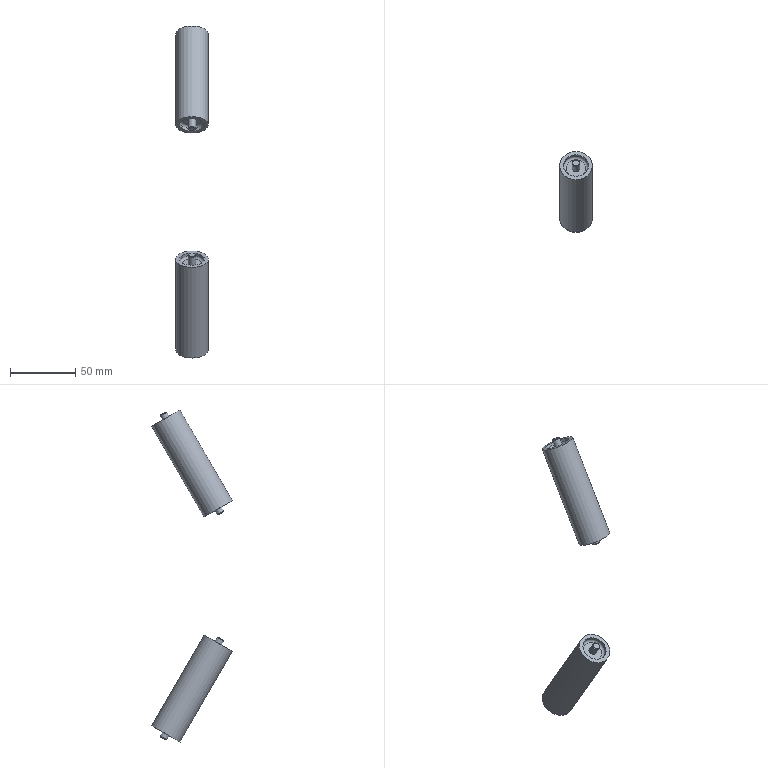Part | STEP file | Idler | 2 solids | 30 faces | box 25 x 61.651 x 253.902 mm | volume 75095 mm3 | plane 12 | cylinder 10 | cone 4 | torus 4 | commonest cylinder face diameters 6 x4 19 x4 25 x2
STEP:
#1=CARTESIAN_POINT('',(0.09843,3.566,-4.888));
#2=VERTEX_POINT('',#1);
#3=CARTESIAN_POINT('',(0.,3.566,-4.888));
#4=DIRECTION('',(0.,0.5,-0.866));
#5=DIRECTION('',(-1.,0.,0.));
#6=AXIS2_PLACEMENT_3D('',#3,#4,#5);
#7=CIRCLE('',#6,0.09843);
#8=EDGE_CURVE('',#2,#2,#7,.T.);
#9=ORIENTED_EDGE('',*,*,#8,.F.);
#10=CARTESIAN_POINT('',(0.1181,3.557,-4.871));
#11=VERTEX_POINT('',#10);
#12=CARTESIAN_POINT('',(0.1083,3.562,-4.88));
#13=DIRECTION('',(0.7071,-0.3536,0.6124));
#14=VECTOR('',#13,0.1083);
#15=LINE('',#12,#14);
#16=EDGE_CURVE('',#2,#11,#15,.T.);
#17=ORIENTED_EDGE('',*,*,#16,.T.);
#18=CARTESIAN_POINT('',(-0.1181,3.557,-4.871));
#19=VERTEX_POINT('',#18);
#20=CARTESIAN_POINT('',(0.,3.557,-4.871));
#21=DIRECTION('',(0.,-0.5,0.866));
#22=DIRECTION('',(-1.,0.,0.));
#23=AXIS2_PLACEMENT_3D('',#20,#21,#22);
#24=CIRCLE('',#23,0.1181);
#25=EDGE_CURVE('',#19,#11,#24,.T.);
#26=ORIENTED_EDGE('',*,*,#25,.F.);
#27=CARTESIAN_POINT('',(0.,3.557,-4.871));
#28=DIRECTION('',(0.,-0.5,0.866));
#29=DIRECTION('',(-1.,0.,0.));
#30=AXIS2_PLACEMENT_3D('',#27,#28,#29);
#31=CIRCLE('',#30,0.1181);
#32=EDGE_CURVE('',#11,#19,#31,.T.);
#33=ORIENTED_EDGE('',*,*,#32,.F.);
#34=ORIENTED_EDGE('',*,*,#16,.F.);
#35=EDGE_LOOP('',(#9,#17,#26,#33,#34));
#36=FACE_OUTER_BOUND('',#35,.T.);
#37=CARTESIAN_POINT('',(0.,3.562,-4.88));
#38=DIRECTION('',(0.,-0.5,0.866));
#39=DIRECTION('',(-1.,0.,0.));
#40=AXIS2_PLACEMENT_3D('',#37,#38,#39);
#41=CONICAL_SURFACE('',#40,0.1083,0.7854);
#42=ADVANCED_FACE('',(#36),#41,.T.);
#43=ORIENTED_EDGE('',*,*,#32,.T.);
#44=CARTESIAN_POINT('',(-0.1181,3.409,-4.616));
#45=VERTEX_POINT('',#44);
#46=CARTESIAN_POINT('',(-0.1181,3.409,-4.616));
#47=DIRECTION('',(0.,-0.5,0.866));
#48=VECTOR('',#47,0.1181);
#49=LINE('',#46,#48);
#50=EDGE_CURVE('',#19,#45,#49,.T.);
#51=ORIENTED_EDGE('',*,*,#50,.T.);
#52=CARTESIAN_POINT('',(0.,3.409,-4.616));
#53=DIRECTION('',(0.,-0.5,0.866));
#54=DIRECTION('',(1.,0.,0.));
#55=AXIS2_PLACEMENT_3D('',#52,#53,#54);
#56=CIRCLE('',#55,0.1181);
#57=EDGE_CURVE('',#45,#45,#56,.T.);
#58=ORIENTED_EDGE('',*,*,#57,.F.);
#59=ORIENTED_EDGE('',*,*,#50,.F.);
#60=ORIENTED_EDGE('',*,*,#25,.T.);
#61=EDGE_LOOP('',(#43,#51,#58,#59,#60));
#62=FACE_OUTER_BOUND('',#61,.T.);
#63=CARTESIAN_POINT('',(0.,3.409,-4.616));
#64=DIRECTION('',(0.,-0.5,0.866));
#65=DIRECTION('',(1.,0.,0.));
#66=AXIS2_PLACEMENT_3D('',#63,#64,#65);
#67=CYLINDRICAL_SURFACE('',#66,0.1181);
#68=ADVANCED_FACE('',(#62),#67,.T.);
#69=ORIENTED_EDGE('',*,*,#8,.T.);
#70=EDGE_LOOP('',(#69));
#71=FACE_OUTER_BOUND('',#70,.T.);
#72=CARTESIAN_POINT('',(0.,3.566,-4.888));
#73=DIRECTION('',(0.,-0.5,0.866));
#74=DIRECTION('',(1.,0.,0.));
#75=AXIS2_PLACEMENT_3D('',#72,#73,#74);
#76=PLANE('',#75);
#77=ADVANCED_FACE('',(#71),#76,.F.);
#78=CARTESIAN_POINT('',(-0.09843,1.834,-1.888));
#79=VERTEX_POINT('',#78);
#80=CARTESIAN_POINT('',(0.,1.834,-1.888));
#81=DIRECTION('',(0.,-0.5,0.866));
#82=DIRECTION('',(1.,0.,0.));
#83=AXIS2_PLACEMENT_3D('',#80,#81,#82);
#84=CIRCLE('',#83,0.09843);
#85=EDGE_CURVE('',#79,#79,#84,.T.);
#86=ORIENTED_EDGE('',*,*,#85,.F.);
#87=CARTESIAN_POINT('',(-0.1181,1.844,-1.905));
#88=VERTEX_POINT('',#87);
#89=CARTESIAN_POINT('',(-0.1083,1.839,-1.897));
#90=DIRECTION('',(-0.7071,0.3536,-0.6124));
#91=VECTOR('',#90,0.1083);
#92=LINE('',#89,#91);
#93=EDGE_CURVE('',#79,#88,#92,.T.);
#94=ORIENTED_EDGE('',*,*,#93,.T.);
#95=CARTESIAN_POINT('',(0.1181,1.844,-1.905));
#96=VERTEX_POINT('',#95);
#97=CARTESIAN_POINT('',(0.,1.844,-1.905));
#98=DIRECTION('',(0.,0.5,-0.866));
#99=DIRECTION('',(1.,0.,0.));
#100=AXIS2_PLACEMENT_3D('',#97,#98,#99);
#101=CIRCLE('',#100,0.1181);
#102=EDGE_CURVE('',#96,#88,#101,.T.);
#103=ORIENTED_EDGE('',*,*,#102,.F.);
#104=CARTESIAN_POINT('',(0.,1.844,-1.905));
#105=DIRECTION('',(0.,0.5,-0.866));
#106=DIRECTION('',(1.,0.,0.));
#107=AXIS2_PLACEMENT_3D('',#104,#105,#106);
#108=CIRCLE('',#107,0.1181);
#109=EDGE_CURVE('',#88,#96,#108,.T.);
#110=ORIENTED_EDGE('',*,*,#109,.F.);
#111=ORIENTED_EDGE('',*,*,#93,.F.);
#112=EDGE_LOOP('',(#86,#94,#103,#110,#111));
#113=FACE_OUTER_BOUND('',#112,.T.);
#114=CARTESIAN_POINT('',(0.,1.839,-1.897));
#115=DIRECTION('',(0.,0.5,-0.866));
#116=DIRECTION('',(1.,0.,0.));
#117=AXIS2_PLACEMENT_3D('',#114,#115,#116);
#118=CONICAL_SURFACE('',#117,0.1083,0.7854);
#119=ADVANCED_FACE('',(#113),#118,.T.);
#120=ORIENTED_EDGE('',*,*,#109,.T.);
#121=CARTESIAN_POINT('',(0.1181,1.992,-2.161));
#122=VERTEX_POINT('',#121);
#123=CARTESIAN_POINT('',(0.1181,1.992,-2.161));
#124=DIRECTION('',(0.,0.5,-0.866));
#125=VECTOR('',#124,0.1181);
#126=LINE('',#123,#125);
#127=EDGE_CURVE('',#96,#122,#126,.T.);
#128=ORIENTED_EDGE('',*,*,#127,.T.);
#129=CARTESIAN_POINT('',(0.,1.992,-2.161));
#130=DIRECTION('',(0.,0.5,-0.866));
#131=DIRECTION('',(-1.,0.,0.));
#132=AXIS2_PLACEMENT_3D('',#129,#130,#131);
#133=CIRCLE('',#132,0.1181);
#134=EDGE_CURVE('',#122,#122,#133,.T.);
#135=ORIENTED_EDGE('',*,*,#134,.F.);
#136=ORIENTED_EDGE('',*,*,#127,.F.);
#137=ORIENTED_EDGE('',*,*,#102,.T.);
#138=EDGE_LOOP('',(#120,#128,#135,#136,#137));
#139=FACE_OUTER_BOUND('',#138,.T.);
#140=CARTESIAN_POINT('',(0.,1.992,-2.161));
#141=DIRECTION('',(0.,0.5,-0.866));
#142=DIRECTION('',(-1.,0.,0.));
#143=AXIS2_PLACEMENT_3D('',#140,#141,#142);
#144=CYLINDRICAL_SURFACE('',#143,0.1181);
#145=ADVANCED_FACE('',(#139),#144,.T.);
#146=ORIENTED_EDGE('',*,*,#85,.T.);
#147=EDGE_LOOP('',(#146));
#148=FACE_OUTER_BOUND('',#147,.T.);
#149=CARTESIAN_POINT('',(0.,1.834,-1.888));
#150=DIRECTION('',(0.,0.5,-0.866));
#151=DIRECTION('',(-1.,0.,0.));
#152=AXIS2_PLACEMENT_3D('',#149,#150,#151);
#153=PLANE('',#152);
#154=ADVANCED_FACE('',(#148),#153,.F.);
#155=CARTESIAN_POINT('',(-0.374,3.448,-4.684));
#156=VERTEX_POINT('',#155);
#157=CARTESIAN_POINT('',(0.374,3.448,-4.684));
#158=VERTEX_POINT('',#157);
#159=CARTESIAN_POINT('',(0.,3.448,-4.684));
#160=DIRECTION('',(0.,-0.5,0.866));
#161=DIRECTION('',(1.,0.,0.));
#162=AXIS2_PLACEMENT_3D('',#159,#160,#161);
#163=CIRCLE('',#162,0.374);
#164=EDGE_CURVE('',#156,#158,#163,.T.);
#165=ORIENTED_EDGE('',*,*,#164,.F.);
#166=CARTESIAN_POINT('',(-0.2953,3.409,-4.616));
#167=VERTEX_POINT('',#166);
#168=CARTESIAN_POINT('',(-0.2953,3.448,-4.684));
#169=DIRECTION('',(0.,0.866,0.5));
#170=DIRECTION('',(-1.,0.,0.));
#171=AXIS2_PLACEMENT_3D('',#168,#169,#170);
#172=CIRCLE('',#171,0.07874);
#173=EDGE_CURVE('',#156,#167,#172,.T.);
#174=ORIENTED_EDGE('',*,*,#173,.T.);
#175=CARTESIAN_POINT('',(0.,3.409,-4.616));
#176=DIRECTION('',(0.,0.5,-0.866));
#177=DIRECTION('',(1.,0.,0.));
#178=AXIS2_PLACEMENT_3D('',#175,#176,#177);
#179=CIRCLE('',#178,0.2953);
#180=EDGE_CURVE('',#167,#167,#179,.T.);
#181=ORIENTED_EDGE('',*,*,#180,.F.);
#182=ORIENTED_EDGE('',*,*,#173,.F.);
#183=CARTESIAN_POINT('',(0.,3.448,-4.684));
#184=DIRECTION('',(0.,-0.5,0.866));
#185=DIRECTION('',(1.,0.,0.));
#186=AXIS2_PLACEMENT_3D('',#183,#184,#185);
#187=CIRCLE('',#186,0.374);
#188=EDGE_CURVE('',#158,#156,#187,.T.);
#189=ORIENTED_EDGE('',*,*,#188,.F.);
#190=EDGE_LOOP('',(#165,#174,#181,#182,#189));
#191=FACE_OUTER_BOUND('',#190,.T.);
#192=CARTESIAN_POINT('',(0.,3.448,-4.684));
#193=DIRECTION('',(0.,-0.5,0.866));
#194=DIRECTION('',(1.,0.,0.));
#195=AXIS2_PLACEMENT_3D('',#192,#193,#194);
#196=TOROIDAL_SURFACE('',#195,0.2953,0.07874);
#197=ADVANCED_FACE('',(#191),#196,.F.);
#198=CARTESIAN_POINT('',(0.374,3.488,-4.752));
#199=VERTEX_POINT('',#198);
#200=CARTESIAN_POINT('',(0.,3.488,-4.752));
#201=DIRECTION('',(0.,-0.5,0.866));
#202=DIRECTION('',(-1.,0.,0.));
#203=AXIS2_PLACEMENT_3D('',#200,#201,#202);
#204=CIRCLE('',#203,0.374);
#205=EDGE_CURVE('',#199,#199,#204,.T.);
#206=ORIENTED_EDGE('',*,*,#205,.F.);
#207=CARTESIAN_POINT('',(0.374,3.488,-4.752));
#208=DIRECTION('',(0.,-0.5,0.866));
#209=VECTOR('',#208,0.374);
#210=LINE('',#207,#209);
#211=EDGE_CURVE('',#199,#158,#210,.T.);
#212=ORIENTED_EDGE('',*,*,#211,.T.);
#213=ORIENTED_EDGE('',*,*,#188,.T.);
#214=ORIENTED_EDGE('',*,*,#164,.T.);
#215=ORIENTED_EDGE('',*,*,#211,.F.);
#216=EDGE_LOOP('',(#206,#212,#213,#214,#215));
#217=FACE_OUTER_BOUND('',#216,.T.);
#218=CARTESIAN_POINT('',(0.,3.488,-4.752));
#219=DIRECTION('',(0.,-0.5,0.866));
#220=DIRECTION('',(-1.,0.,0.));
#221=AXIS2_PLACEMENT_3D('',#218,#219,#220);
#222=CYLINDRICAL_SURFACE('',#221,0.374);
#223=ADVANCED_FACE('',(#217),#222,.F.);
#224=ORIENTED_EDGE('',*,*,#180,.T.);
#225=EDGE_LOOP('',(#224));
#226=FACE_OUTER_BOUND('',#225,.T.);
#227=ORIENTED_EDGE('',*,*,#57,.T.);
#228=EDGE_LOOP('',(#227));
#229=FACE_BOUND('',#228,.T.);
#230=CARTESIAN_POINT('',(0.,3.409,-4.616));
#231=DIRECTION('',(0.,0.5,-0.866));
#232=DIRECTION('',(-1.,0.,0.));
#233=AXIS2_PLACEMENT_3D('',#230,#231,#232);
#234=PLANE('',#233);
#235=ADVANCED_FACE('',(#226,#229),#234,.T.);
#236=CARTESIAN_POINT('',(-0.374,1.952,-2.093));
#237=VERTEX_POINT('',#236);
#238=CARTESIAN_POINT('',(0.374,1.952,-2.093));
#239=VERTEX_POINT('',#238);
#240=CARTESIAN_POINT('',(0.,1.952,-2.093));
#241=DIRECTION('',(0.,-0.5,0.866));
#242=DIRECTION('',(1.,0.,0.));
#243=AXIS2_PLACEMENT_3D('',#240,#241,#242);
#244=CIRCLE('',#243,0.374);
#245=EDGE_CURVE('',#237,#239,#244,.T.);
#246=ORIENTED_EDGE('',*,*,#245,.T.);
#247=CARTESIAN_POINT('',(0.,1.952,-2.093));
#248=DIRECTION('',(0.,-0.5,0.866));
#249=DIRECTION('',(1.,0.,0.));
#250=AXIS2_PLACEMENT_3D('',#247,#248,#249);
#251=CIRCLE('',#250,0.374);
#252=EDGE_CURVE('',#239,#237,#251,.T.);
#253=ORIENTED_EDGE('',*,*,#252,.T.);
#254=CARTESIAN_POINT('',(-0.2953,1.992,-2.161));
#255=VERTEX_POINT('',#254);
#256=CARTESIAN_POINT('',(-0.2953,1.952,-2.093));
#257=DIRECTION('',(0.,-0.866,-0.5));
#258=DIRECTION('',(-1.,0.,0.));
#259=AXIS2_PLACEMENT_3D('',#256,#257,#258);
#260=CIRCLE('',#259,0.07874);
#261=EDGE_CURVE('',#237,#255,#260,.T.);
#262=ORIENTED_EDGE('',*,*,#261,.T.);
#263=CARTESIAN_POINT('',(0.,1.992,-2.161));
#264=DIRECTION('',(0.,0.5,-0.866));
#265=DIRECTION('',(1.,0.,0.));
#266=AXIS2_PLACEMENT_3D('',#263,#264,#265);
#267=CIRCLE('',#266,0.2953);
#268=EDGE_CURVE('',#255,#255,#267,.T.);
#269=ORIENTED_EDGE('',*,*,#268,.T.);
#270=ORIENTED_EDGE('',*,*,#261,.F.);
#271=EDGE_LOOP('',(#246,#253,#262,#269,#270));
#272=FACE_OUTER_BOUND('',#271,.T.);
#273=CARTESIAN_POINT('',(0.,1.952,-2.093));
#274=DIRECTION('',(0.,0.5,-0.866));
#275=DIRECTION('',(1.,0.,0.));
#276=AXIS2_PLACEMENT_3D('',#273,#274,#275);
#277=TOROIDAL_SURFACE('',#276,0.2953,0.07874);
#278=ADVANCED_FACE('',(#272),#277,.F.);
#279=CARTESIAN_POINT('',(0.374,1.913,-2.024));
#280=VERTEX_POINT('',#279);
#281=CARTESIAN_POINT('',(0.,1.913,-2.024));
#282=DIRECTION('',(0.,0.5,-0.866));
#283=DIRECTION('',(-1.,0.,0.));
#284=AXIS2_PLACEMENT_3D('',#281,#282,#283);
#285=CIRCLE('',#284,0.374);
#286=EDGE_CURVE('',#280,#280,#285,.T.);
#287=ORIENTED_EDGE('',*,*,#286,.F.);
#288=CARTESIAN_POINT('',(0.374,1.913,-2.024));
#289=DIRECTION('',(0.,0.5,-0.866));
#290=VECTOR('',#289,0.374);
#291=LINE('',#288,#290);
#292=EDGE_CURVE('',#280,#239,#291,.T.);
#293=ORIENTED_EDGE('',*,*,#292,.T.);
#294=ORIENTED_EDGE('',*,*,#245,.F.);
#295=ORIENTED_EDGE('',*,*,#252,.F.);
#296=ORIENTED_EDGE('',*,*,#292,.F.);
#297=EDGE_LOOP('',(#287,#293,#294,#295,#296));
#298=FACE_OUTER_BOUND('',#297,.T.);
#299=CARTESIAN_POINT('',(0.,1.913,-2.024));
#300=DIRECTION('',(0.,-0.5,0.866));
#301=DIRECTION('',(-1.,0.,0.));
#302=AXIS2_PLACEMENT_3D('',#299,#300,#301);
#303=CYLINDRICAL_SURFACE('',#302,0.374);
#304=ADVANCED_FACE('',(#298),#303,.F.);
#305=ORIENTED_EDGE('',*,*,#268,.F.);
#306=EDGE_LOOP('',(#305));
#307=FACE_OUTER_BOUND('',#306,.T.);
#308=ORIENTED_EDGE('',*,*,#134,.T.);
#309=EDGE_LOOP('',(#308));
#310=FACE_BOUND('',#309,.T.);
#311=CARTESIAN_POINT('',(0.,1.992,-2.161));
#312=DIRECTION('',(0.,0.5,-0.866));
#313=DIRECTION('',(-1.,0.,0.));
#314=AXIS2_PLACEMENT_3D('',#311,#312,#313);
#315=PLANE('',#314);
#316=ADVANCED_FACE('',(#307,#310),#315,.F.);
#317=CARTESIAN_POINT('',(0.,1.487,-2.27));
#318=VERTEX_POINT('',#317);
#319=CARTESIAN_POINT('',(0.,1.913,-2.024));
#320=DIRECTION('',(0.,0.5,-0.866));
#321=DIRECTION('',(1.,0.,0.));
#322=AXIS2_PLACEMENT_3D('',#319,#320,#321);
#323=CIRCLE('',#322,0.4921);
#324=EDGE_CURVE('',#318,#318,#323,.T.);
#325=ORIENTED_EDGE('',*,*,#324,.F.);
#326=EDGE_LOOP('',(#325));
#327=FACE_OUTER_BOUND('',#326,.T.);
#328=ORIENTED_EDGE('',*,*,#286,.T.);
#329=EDGE_LOOP('',(#328));
#330=FACE_BOUND('',#329,.T.);
#331=CARTESIAN_POINT('',(0.,1.913,-2.024));
#332=DIRECTION('',(0.,0.5,-0.866));
#333=DIRECTION('',(-1.,0.,0.));
#334=AXIS2_PLACEMENT_3D('',#331,#332,#333);
#335=PLANE('',#334);
#336=ADVANCED_FACE('',(#327,#330),#335,.F.);
#337=CARTESIAN_POINT('',(0.,3.062,-4.998));
#338=VERTEX_POINT('',#337);
#339=CARTESIAN_POINT('',(0.,3.488,-4.752));
#340=DIRECTION('',(0.,0.5,-0.866));
#341=DIRECTION('',(1.,0.,0.));
#342=AXIS2_PLACEMENT_3D('',#339,#340,#341);
#343=CIRCLE('',#342,0.4921);
#344=EDGE_CURVE('',#338,#338,#343,.T.);
#345=ORIENTED_EDGE('',*,*,#344,.T.);
#346=EDGE_LOOP('',(#345));
#347=FACE_OUTER_BOUND('',#346,.T.);
#348=ORIENTED_EDGE('',*,*,#205,.T.);
#349=EDGE_LOOP('',(#348));
#350=FACE_BOUND('',#349,.T.);
#351=CARTESIAN_POINT('',(0.,3.914,-4.506));
#352=DIRECTION('',(0.,-0.5,0.866));
#353=DIRECTION('',(1.,0.,0.));
#354=AXIS2_PLACEMENT_3D('',#351,#352,#353);
#355=PLANE('',#354);
#356=ADVANCED_FACE('',(#347,#350),#355,.F.);
#357=ORIENTED_EDGE('',*,*,#324,.T.);
#358=CARTESIAN_POINT('',(0.,2.274,-3.634));
#359=DIRECTION('',(0.,0.5,-0.866));
#360=VECTOR('',#359,0.4921);
#361=LINE('',#358,#360);
#362=EDGE_CURVE('',#318,#338,#361,.T.);
#363=ORIENTED_EDGE('',*,*,#362,.T.);
#364=ORIENTED_EDGE('',*,*,#344,.F.);
#365=ORIENTED_EDGE('',*,*,#362,.F.);
#366=EDGE_LOOP('',(#357,#363,#364,#365));
#367=FACE_OUTER_BOUND('',#366,.T.);
#368=CARTESIAN_POINT('',(0.,2.7,-3.388));
#369=DIRECTION('',(0.,0.5,-0.866));
#370=DIRECTION('',(0.,0.866,0.5));
#371=AXIS2_PLACEMENT_3D('',#368,#369,#370);
#372=CYLINDRICAL_SURFACE('',#371,0.4921);
#373=ADVANCED_FACE('',(#367),#372,.T.);
#374=CLOSED_SHELL('',(#42,#68,#77,#119,#145,#154,#197,#223,#235,#278,#304,#316,#336,#356,#373));
#375=MANIFOLD_SOLID_BREP('',#374);
#376=CARTESIAN_POINT('',(0.09843,3.566,4.888));
#377=VERTEX_POINT('',#376);
#378=CARTESIAN_POINT('',(0.,3.566,4.888));
#379=DIRECTION('',(0.,-0.5,-0.866));
#380=DIRECTION('',(-1.,0.,0.));
#381=AXIS2_PLACEMENT_3D('',#378,#379,#380);
#382=CIRCLE('',#381,0.09843);
#383=EDGE_CURVE('',#377,#377,#382,.T.);
#384=ORIENTED_EDGE('',*,*,#383,.T.);
#385=CARTESIAN_POINT('',(0.1181,3.557,4.871));
#386=VERTEX_POINT('',#385);
#387=CARTESIAN_POINT('',(0.1083,3.562,4.88));
#388=DIRECTION('',(0.7071,-0.3536,-0.6124));
#389=VECTOR('',#388,0.1083);
#390=LINE('',#387,#389);
#391=EDGE_CURVE('',#377,#386,#390,.T.);
#392=ORIENTED_EDGE('',*,*,#391,.T.);
#393=CARTESIAN_POINT('',(-0.1181,3.557,4.871));
#394=VERTEX_POINT('',#393);
#395=CARTESIAN_POINT('',(0.,3.557,4.871));
#396=DIRECTION('',(0.,0.5,0.866));
#397=DIRECTION('',(-1.,0.,0.));
#398=AXIS2_PLACEMENT_3D('',#395,#396,#397);
#399=CIRCLE('',#398,0.1181);
#400=EDGE_CURVE('',#386,#394,#399,.T.);
#401=ORIENTED_EDGE('',*,*,#400,.T.);
#402=CARTESIAN_POINT('',(0.,3.557,4.871));
#403=DIRECTION('',(0.,0.5,0.866));
#404=DIRECTION('',(-1.,0.,0.));
#405=AXIS2_PLACEMENT_3D('',#402,#403,#404);
#406=CIRCLE('',#405,0.1181);
#407=EDGE_CURVE('',#394,#386,#406,.T.);
#408=ORIENTED_EDGE('',*,*,#407,.T.);
#409=ORIENTED_EDGE('',*,*,#391,.F.);
#410=EDGE_LOOP('',(#384,#392,#401,#408,#409));
#411=FACE_OUTER_BOUND('',#410,.T.);
#412=CARTESIAN_POINT('',(0.,3.562,4.88));
#413=DIRECTION('',(0.,-0.5,-0.866));
#414=DIRECTION('',(-1.,0.,0.));
#415=AXIS2_PLACEMENT_3D('',#412,#413,#414);
#416=CONICAL_SURFACE('',#415,0.1083,0.7854);
#417=ADVANCED_FACE('',(#411),#416,.T.);
#418=ORIENTED_EDGE('',*,*,#400,.F.);
#419=ORIENTED_EDGE('',*,*,#407,.F.);
#420=CARTESIAN_POINT('',(-0.1181,3.409,4.616));
#421=VERTEX_POINT('',#420);
#422=CARTESIAN_POINT('',(-0.1181,3.409,4.616));
#423=DIRECTION('',(0.,-0.5,-0.866));
#424=VECTOR('',#423,0.1181);
#425=LINE('',#422,#424);
#426=EDGE_CURVE('',#394,#421,#425,.T.);
#427=ORIENTED_EDGE('',*,*,#426,.T.);
#428=CARTESIAN_POINT('',(0.,3.409,4.616));
#429=DIRECTION('',(0.,-0.5,-0.866));
#430=DIRECTION('',(1.,0.,0.));
#431=AXIS2_PLACEMENT_3D('',#428,#429,#430);
#432=CIRCLE('',#431,0.1181);
#433=EDGE_CURVE('',#421,#421,#432,.T.);
#434=ORIENTED_EDGE('',*,*,#433,.F.);
#435=ORIENTED_EDGE('',*,*,#426,.F.);
#436=EDGE_LOOP('',(#418,#419,#427,#434,#435));
#437=FACE_OUTER_BOUND('',#436,.T.);
#438=CARTESIAN_POINT('',(0.,3.409,4.616));
#439=DIRECTION('',(0.,0.5,0.866));
#440=DIRECTION('',(1.,0.,0.));
#441=AXIS2_PLACEMENT_3D('',#438,#439,#440);
#442=CYLINDRICAL_SURFACE('',#441,0.1181);
#443=ADVANCED_FACE('',(#437),#442,.T.);
#444=ORIENTED_EDGE('',*,*,#383,.F.);
#445=EDGE_LOOP('',(#444));
#446=FACE_OUTER_BOUND('',#445,.T.);
#447=CARTESIAN_POINT('',(0.,3.566,4.888));
#448=DIRECTION('',(0.,0.5,0.866));
#449=DIRECTION('',(1.,0.,0.));
#450=AXIS2_PLACEMENT_3D('',#447,#448,#449);
#451=PLANE('',#450);
#452=ADVANCED_FACE('',(#446),#451,.T.);
#453=CARTESIAN_POINT('',(-0.09843,1.834,1.888));
#454=VERTEX_POINT('',#453);
#455=CARTESIAN_POINT('',(0.,1.834,1.888));
#456=DIRECTION('',(0.,0.5,0.866));
#457=DIRECTION('',(1.,0.,0.));
#458=AXIS2_PLACEMENT_3D('',#455,#456,#457);
#459=CIRCLE('',#458,0.09843);
#460=EDGE_CURVE('',#454,#454,#459,.T.);
#461=ORIENTED_EDGE('',*,*,#460,.T.);
#462=CARTESIAN_POINT('',(-0.1181,1.844,1.905));
#463=VERTEX_POINT('',#462);
#464=CARTESIAN_POINT('',(-0.1083,1.839,1.897));
#465=DIRECTION('',(-0.7071,0.3536,0.6124));
#466=VECTOR('',#465,0.1083);
#467=LINE('',#464,#466);
#468=EDGE_CURVE('',#454,#463,#467,.T.);
#469=ORIENTED_EDGE('',*,*,#468,.T.);
#470=CARTESIAN_POINT('',(0.1181,1.844,1.905));
#471=VERTEX_POINT('',#470);
#472=CARTESIAN_POINT('',(0.,1.844,1.905));
#473=DIRECTION('',(0.,-0.5,-0.866));
#474=DIRECTION('',(1.,0.,0.));
#475=AXIS2_PLACEMENT_3D('',#472,#473,#474);
#476=CIRCLE('',#475,0.1181);
#477=EDGE_CURVE('',#463,#471,#476,.T.);
#478=ORIENTED_EDGE('',*,*,#477,.T.);
#479=CARTESIAN_POINT('',(0.,1.844,1.905));
#480=DIRECTION('',(0.,-0.5,-0.866));
#481=DIRECTION('',(1.,0.,0.));
#482=AXIS2_PLACEMENT_3D('',#479,#480,#481);
#483=CIRCLE('',#482,0.1181);
#484=EDGE_CURVE('',#471,#463,#483,.T.);
#485=ORIENTED_EDGE('',*,*,#484,.T.);
#486=ORIENTED_EDGE('',*,*,#468,.F.);
#487=EDGE_LOOP('',(#461,#469,#478,#485,#486));
#488=FACE_OUTER_BOUND('',#487,.T.);
#489=CARTESIAN_POINT('',(0.,1.839,1.897));
#490=DIRECTION('',(0.,0.5,0.866));
#491=DIRECTION('',(1.,0.,0.));
#492=AXIS2_PLACEMENT_3D('',#489,#490,#491);
#493=CONICAL_SURFACE('',#492,0.1083,0.7854);
#494=ADVANCED_FACE('',(#488),#493,.T.);
#495=ORIENTED_EDGE('',*,*,#477,.F.);
#496=ORIENTED_EDGE('',*,*,#484,.F.);
#497=CARTESIAN_POINT('',(0.1181,1.992,2.161));
#498=VERTEX_POINT('',#497);
#499=CARTESIAN_POINT('',(0.1181,1.992,2.161));
#500=DIRECTION('',(0.,0.5,0.866));
#501=VECTOR('',#500,0.1181);
#502=LINE('',#499,#501);
#503=EDGE_CURVE('',#471,#498,#502,.T.);
#504=ORIENTED_EDGE('',*,*,#503,.T.);
#505=CARTESIAN_POINT('',(0.,1.992,2.161));
#506=DIRECTION('',(0.,0.5,0.866));
#507=DIRECTION('',(-1.,0.,0.));
#508=AXIS2_PLACEMENT_3D('',#505,#506,#507);
#509=CIRCLE('',#508,0.1181);
#510=EDGE_CURVE('',#498,#498,#509,.T.);
#511=ORIENTED_EDGE('',*,*,#510,.F.);
#512=ORIENTED_EDGE('',*,*,#503,.F.);
#513=EDGE_LOOP('',(#495,#496,#504,#511,#512));
#514=FACE_OUTER_BOUND('',#513,.T.);
#515=CARTESIAN_POINT('',(0.,1.992,2.161));
#516=DIRECTION('',(0.,-0.5,-0.866));
#517=DIRECTION('',(-1.,0.,0.));
#518=AXIS2_PLACEMENT_3D('',#515,#516,#517);
#519=CYLINDRICAL_SURFACE('',#518,0.1181);
#520=ADVANCED_FACE('',(#514),#519,.T.);
#521=ORIENTED_EDGE('',*,*,#460,.F.);
#522=EDGE_LOOP('',(#521));
#523=FACE_OUTER_BOUND('',#522,.T.);
#524=CARTESIAN_POINT('',(0.,1.834,1.888));
#525=DIRECTION('',(0.,-0.5,-0.866));
#526=DIRECTION('',(-1.,0.,0.));
#527=AXIS2_PLACEMENT_3D('',#524,#525,#526);
#528=PLANE('',#527);
#529=ADVANCED_FACE('',(#523),#528,.T.);
#530=CARTESIAN_POINT('',(-0.374,3.448,4.684));
#531=VERTEX_POINT('',#530);
#532=CARTESIAN_POINT('',(0.374,3.448,4.684));
#533=VERTEX_POINT('',#532);
#534=CARTESIAN_POINT('',(0.,3.448,4.684));
#535=DIRECTION('',(0.,0.5,0.866));
#536=DIRECTION('',(1.,0.,0.));
#537=AXIS2_PLACEMENT_3D('',#534,#535,#536);
#538=CIRCLE('',#537,0.374);
#539=EDGE_CURVE('',#531,#533,#538,.T.);
#540=ORIENTED_EDGE('',*,*,#539,.T.);
#541=CARTESIAN_POINT('',(0.,3.448,4.684));
#542=DIRECTION('',(0.,0.5,0.866));
#543=DIRECTION('',(1.,0.,0.));
#544=AXIS2_PLACEMENT_3D('',#541,#542,#543);
#545=CIRCLE('',#544,0.374);
#546=EDGE_CURVE('',#533,#531,#545,.T.);
#547=ORIENTED_EDGE('',*,*,#546,.T.);
#548=CARTESIAN_POINT('',(-0.2953,3.409,4.616));
#549=VERTEX_POINT('',#548);
#550=CARTESIAN_POINT('',(-0.2953,3.448,4.684));
#551=DIRECTION('',(0.,-0.866,0.5));
#552=DIRECTION('',(-1.,0.,0.));
#553=AXIS2_PLACEMENT_3D('',#550,#551,#552);
#554=CIRCLE('',#553,0.07874);
#555=EDGE_CURVE('',#531,#549,#554,.T.);
#556=ORIENTED_EDGE('',*,*,#555,.T.);
#557=CARTESIAN_POINT('',(0.,3.409,4.616));
#558=DIRECTION('',(0.,-0.5,-0.866));
#559=DIRECTION('',(1.,0.,0.));
#560=AXIS2_PLACEMENT_3D('',#557,#558,#559);
#561=CIRCLE('',#560,0.2953);
#562=EDGE_CURVE('',#549,#549,#561,.T.);
#563=ORIENTED_EDGE('',*,*,#562,.T.);
#564=ORIENTED_EDGE('',*,*,#555,.F.);
#565=EDGE_LOOP('',(#540,#547,#556,#563,#564));
#566=FACE_OUTER_BOUND('',#565,.T.);
#567=CARTESIAN_POINT('',(0.,3.448,4.684));
#568=DIRECTION('',(0.,-0.5,-0.866));
#569=DIRECTION('',(1.,0.,0.));
#570=AXIS2_PLACEMENT_3D('',#567,#568,#569);
#571=TOROIDAL_SURFACE('',#570,0.2953,0.07874);
#572=ADVANCED_FACE('',(#566),#571,.F.);
#573=CARTESIAN_POINT('',(0.374,3.488,4.752));
#574=VERTEX_POINT('',#573);
#575=CARTESIAN_POINT('',(0.,3.488,4.752));
#576=DIRECTION('',(0.,-0.5,-0.866));
#577=DIRECTION('',(-1.,0.,0.));
#578=AXIS2_PLACEMENT_3D('',#575,#576,#577);
#579=CIRCLE('',#578,0.374);
#580=EDGE_CURVE('',#574,#574,#579,.T.);
#581=ORIENTED_EDGE('',*,*,#580,.F.);
#582=CARTESIAN_POINT('',(0.374,3.488,4.752));
#583=DIRECTION('',(0.,-0.5,-0.866));
#584=VECTOR('',#583,0.374);
#585=LINE('',#582,#584);
#586=EDGE_CURVE('',#574,#533,#585,.T.);
#587=ORIENTED_EDGE('',*,*,#586,.T.);
#588=ORIENTED_EDGE('',*,*,#539,.F.);
#589=ORIENTED_EDGE('',*,*,#546,.F.);
#590=ORIENTED_EDGE('',*,*,#586,.F.);
#591=EDGE_LOOP('',(#581,#587,#588,#589,#590));
#592=FACE_OUTER_BOUND('',#591,.T.);
#593=CARTESIAN_POINT('',(0.,3.488,4.752));
#594=DIRECTION('',(0.,0.5,0.866));
#595=DIRECTION('',(-1.,0.,0.));
#596=AXIS2_PLACEMENT_3D('',#593,#594,#595);
#597=CYLINDRICAL_SURFACE('',#596,0.374);
#598=ADVANCED_FACE('',(#592),#597,.F.);
#599=ORIENTED_EDGE('',*,*,#562,.F.);
#600=EDGE_LOOP('',(#599));
#601=FACE_OUTER_BOUND('',#600,.T.);
#602=ORIENTED_EDGE('',*,*,#433,.T.);
#603=EDGE_LOOP('',(#602));
#604=FACE_BOUND('',#603,.T.);
#605=CARTESIAN_POINT('',(0.,3.409,4.616));
#606=DIRECTION('',(0.,-0.5,-0.866));
#607=DIRECTION('',(-1.,0.,0.));
#608=AXIS2_PLACEMENT_3D('',#605,#606,#607);
#609=PLANE('',#608);
#610=ADVANCED_FACE('',(#601,#604),#609,.F.);
#611=CARTESIAN_POINT('',(-0.2953,1.992,2.161));
#612=VERTEX_POINT('',#611);
#613=CARTESIAN_POINT('',(0.,1.992,2.161));
#614=DIRECTION('',(0.,0.5,0.866));
#615=DIRECTION('',(1.,0.,0.));
#616=AXIS2_PLACEMENT_3D('',#613,#614,#615);
#617=CIRCLE('',#616,0.2953);
#618=EDGE_CURVE('',#612,#612,#617,.T.);
#619=ORIENTED_EDGE('',*,*,#618,.T.);
#620=CARTESIAN_POINT('',(-0.374,1.952,2.093));
#621=VERTEX_POINT('',#620);
#622=CARTESIAN_POINT('',(-0.2953,1.952,2.093));
#623=DIRECTION('',(0.,-0.866,0.5));
#624=DIRECTION('',(-1.,0.,0.));
#625=AXIS2_PLACEMENT_3D('',#622,#623,#624);
#626=CIRCLE('',#625,0.07874);
#627=EDGE_CURVE('',#612,#621,#626,.T.);
#628=ORIENTED_EDGE('',*,*,#627,.T.);
#629=CARTESIAN_POINT('',(0.374,1.952,2.093));
#630=VERTEX_POINT('',#629);
#631=CARTESIAN_POINT('',(0.,1.952,2.093));
#632=DIRECTION('',(0.,-0.5,-0.866));
#633=DIRECTION('',(1.,0.,0.));
#634=AXIS2_PLACEMENT_3D('',#631,#632,#633);
#635=CIRCLE('',#634,0.374);
#636=EDGE_CURVE('',#621,#630,#635,.T.);
#637=ORIENTED_EDGE('',*,*,#636,.T.);
#638=CARTESIAN_POINT('',(0.,1.952,2.093));
#639=DIRECTION('',(0.,-0.5,-0.866));
#640=DIRECTION('',(1.,0.,0.));
#641=AXIS2_PLACEMENT_3D('',#638,#639,#640);
#642=CIRCLE('',#641,0.374);
#643=EDGE_CURVE('',#630,#621,#642,.T.);
#644=ORIENTED_EDGE('',*,*,#643,.T.);
#645=ORIENTED_EDGE('',*,*,#627,.F.);
#646=EDGE_LOOP('',(#619,#628,#637,#644,#645));
#647=FACE_OUTER_BOUND('',#646,.T.);
#648=CARTESIAN_POINT('',(0.,1.952,2.093));
#649=DIRECTION('',(0.,0.5,0.866));
#650=DIRECTION('',(1.,0.,0.));
#651=AXIS2_PLACEMENT_3D('',#648,#649,#650);
#652=TOROIDAL_SURFACE('',#651,0.2953,0.07874);
#653=ADVANCED_FACE('',(#647),#652,.F.);
#654=CARTESIAN_POINT('',(0.374,1.913,2.024));
#655=VERTEX_POINT('',#654);
#656=CARTESIAN_POINT('',(0.,1.913,2.024));
#657=DIRECTION('',(0.,0.5,0.866));
#658=DIRECTION('',(-1.,0.,0.));
#659=AXIS2_PLACEMENT_3D('',#656,#657,#658);
#660=CIRCLE('',#659,0.374);
#661=EDGE_CURVE('',#655,#655,#660,.T.);
#662=ORIENTED_EDGE('',*,*,#661,.F.);
#663=CARTESIAN_POINT('',(0.374,1.913,2.024));
#664=DIRECTION('',(0.,0.5,0.866));
#665=VECTOR('',#664,0.374);
#666=LINE('',#663,#665);
#667=EDGE_CURVE('',#655,#630,#666,.T.);
#668=ORIENTED_EDGE('',*,*,#667,.T.);
#669=ORIENTED_EDGE('',*,*,#636,.F.);
#670=ORIENTED_EDGE('',*,*,#643,.F.);
#671=ORIENTED_EDGE('',*,*,#667,.F.);
#672=EDGE_LOOP('',(#662,#668,#669,#670,#671));
#673=FACE_OUTER_BOUND('',#672,.T.);
#674=CARTESIAN_POINT('',(0.,1.913,2.024));
#675=DIRECTION('',(0.,0.5,0.866));
#676=DIRECTION('',(-1.,0.,0.));
#677=AXIS2_PLACEMENT_3D('',#674,#675,#676);
#678=CYLINDRICAL_SURFACE('',#677,0.374);
#679=ADVANCED_FACE('',(#673),#678,.F.);
#680=ORIENTED_EDGE('',*,*,#618,.F.);
#681=EDGE_LOOP('',(#680));
#682=FACE_OUTER_BOUND('',#681,.T.);
#683=ORIENTED_EDGE('',*,*,#510,.T.);
#684=EDGE_LOOP('',(#683));
#685=FACE_BOUND('',#684,.T.);
#686=CARTESIAN_POINT('',(0.,1.992,2.161));
#687=DIRECTION('',(0.,-0.5,-0.866));
#688=DIRECTION('',(-1.,0.,0.));
#689=AXIS2_PLACEMENT_3D('',#686,#687,#688);
#690=PLANE('',#689);
#691=ADVANCED_FACE('',(#682,#685),#690,.T.);
#692=CARTESIAN_POINT('',(0.,1.487,2.27));
#693=VERTEX_POINT('',#692);
#694=CARTESIAN_POINT('',(0.,1.913,2.024));
#695=DIRECTION('',(0.,-0.5,-0.866));
#696=DIRECTION('',(1.,0.,0.));
#697=AXIS2_PLACEMENT_3D('',#694,#695,#696);
#698=CIRCLE('',#697,0.4921);
#699=EDGE_CURVE('',#693,#693,#698,.T.);
#700=ORIENTED_EDGE('',*,*,#699,.T.);
#701=EDGE_LOOP('',(#700));
#702=FACE_OUTER_BOUND('',#701,.T.);
#703=ORIENTED_EDGE('',*,*,#661,.T.);
#704=EDGE_LOOP('',(#703));
#705=FACE_BOUND('',#704,.T.);
#706=CARTESIAN_POINT('',(0.,1.913,2.024));
#707=DIRECTION('',(0.,-0.5,-0.866));
#708=DIRECTION('',(-1.,0.,0.));
#709=AXIS2_PLACEMENT_3D('',#706,#707,#708);
#710=PLANE('',#709);
#711=ADVANCED_FACE('',(#702,#705),#710,.T.);
#712=CARTESIAN_POINT('',(0.,3.062,4.998));
#713=VERTEX_POINT('',#712);
#714=CARTESIAN_POINT('',(0.,3.488,4.752));
#715=DIRECTION('',(0.,-0.5,-0.866));
#716=DIRECTION('',(1.,0.,0.));
#717=AXIS2_PLACEMENT_3D('',#714,#715,#716);
#718=CIRCLE('',#717,0.4921);
#719=EDGE_CURVE('',#713,#713,#718,.T.);
#720=ORIENTED_EDGE('',*,*,#719,.F.);
#721=EDGE_LOOP('',(#720));
#722=FACE_OUTER_BOUND('',#721,.T.);
#723=ORIENTED_EDGE('',*,*,#580,.T.);
#724=EDGE_LOOP('',(#723));
#725=FACE_BOUND('',#724,.T.);
#726=CARTESIAN_POINT('',(0.,3.914,4.506));
#727=DIRECTION('',(0.,0.5,0.866));
#728=DIRECTION('',(1.,0.,0.));
#729=AXIS2_PLACEMENT_3D('',#726,#727,#728);
#730=PLANE('',#729);
#731=ADVANCED_FACE('',(#722,#725),#730,.T.);
#732=ORIENTED_EDGE('',*,*,#699,.F.);
#733=CARTESIAN_POINT('',(0.,2.274,3.634));
#734=DIRECTION('',(0.,0.5,0.866));
#735=VECTOR('',#734,0.4921);
#736=LINE('',#733,#735);
#737=EDGE_CURVE('',#693,#713,#736,.T.);
#738=ORIENTED_EDGE('',*,*,#737,.T.);
#739=ORIENTED_EDGE('',*,*,#719,.T.);
#740=ORIENTED_EDGE('',*,*,#737,.F.);
#741=EDGE_LOOP('',(#732,#738,#739,#740));
#742=FACE_OUTER_BOUND('',#741,.T.);
#743=CARTESIAN_POINT('',(0.,2.7,3.388));
#744=DIRECTION('',(0.,-0.5,-0.866));
#745=DIRECTION('',(0.,0.866,-0.5));
#746=AXIS2_PLACEMENT_3D('',#743,#744,#745);
#747=CYLINDRICAL_SURFACE('',#746,0.4921);
#748=ADVANCED_FACE('',(#742),#747,.T.);
#749=CLOSED_SHELL('',(#417,#443,#452,#494,#520,#529,#572,#598,#610,#653,#679,#691,#711,#731,#748));
#750=MANIFOLD_SOLID_BREP('',#749);
#751=(LENGTH_UNIT()NAMED_UNIT(*)SI_UNIT(.MILLI.,.METRE.));
#752=LENGTH_MEASURE_WITH_UNIT(LENGTH_MEASURE(25.4),#751);
#753=DIMENSIONAL_EXPONENTS(1.,0.,0.,0.,0.,0.,0.);
#754=(CONVERSION_BASED_UNIT('inch',#752)LENGTH_UNIT()NAMED_UNIT(#753));
#755=UNCERTAINTY_MEASURE_WITH_UNIT(LENGTH_MEASURE(0.0003937),#754,'','');
#756=(NAMED_UNIT(*)PLANE_ANGLE_UNIT()SI_UNIT($,.RADIAN.));
#757=(NAMED_UNIT(*)SI_UNIT($,.STERADIAN.)SOLID_ANGLE_UNIT());
#758=(GEOMETRIC_REPRESENTATION_CONTEXT(3)GLOBAL_UNCERTAINTY_ASSIGNED_CONTEXT((#755))GLOBAL_UNIT_ASSIGNED_CONTEXT((#754,#756,#757))REPRESENTATION_CONTEXT('',''));
#759=ADVANCED_BREP_SHAPE_REPRESENTATION('',(#375,#750),#758);